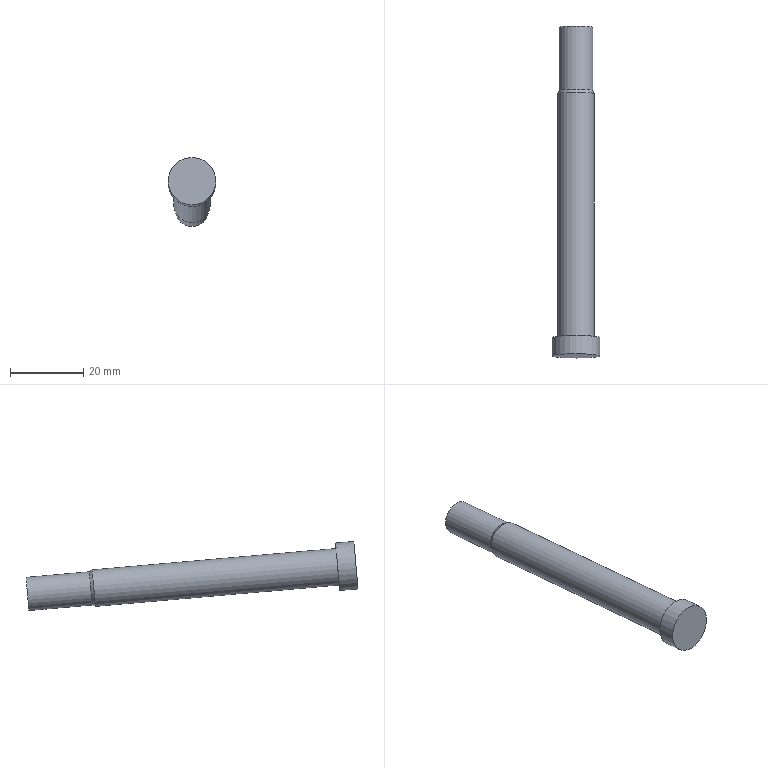Part | NX | features SPAS 10-80-7.100 2 | 1 solid | 7 faces | box 13 x 90.621 x 18.852 mm | volume 7099 mm3 | plane 3 | cylinder 3 | torus 1 | commonest cylinder face diameters 9.1 x1 10 x1 13 x1
STEP:
#1=CARTESIAN_POINT('',(-694.42,-51.795,-32.008));
#2=VERTEX_POINT('',#1);
#3=CARTESIAN_POINT('',(-694.42,-52.191,-36.54));
#4=DIRECTION('',(0.,0.9962,-0.08716));
#5=DIRECTION('',(0.,0.08716,0.9962));
#6=AXIS2_PLACEMENT_3D('',#3,#4,#5);
#7=CIRCLE('',#6,4.55);
#8=EDGE_CURVE('',#2,#2,#7,.F.);
#9=ORIENTED_EDGE('',*,*,#8,.F.);
#10=EDGE_LOOP('',(#9));
#11=FACE_BOUND('',#10,.T.);
#12=CARTESIAN_POINT('',(-694.42,-52.191,-36.54));
#13=DIRECTION('',(0.,0.9962,-0.08716));
#14=DIRECTION('',(0.,0.08716,0.9962));
#15=AXIS2_PLACEMENT_3D('',#12,#13,#14);
#16=PLANE('',#15);
#17=ADVANCED_FACE('',(#11),#16,.T.);
#18=CARTESIAN_POINT('',(-694.42,-69.087,-30.495));
#19=VERTEX_POINT('',#18);
#20=CARTESIAN_POINT('',(-694.42,-69.484,-35.027));
#21=DIRECTION('',(0.,0.9962,-0.08716));
#22=DIRECTION('',(0.,0.08716,0.9962));
#23=AXIS2_PLACEMENT_3D('',#20,#21,#22);
#24=CIRCLE('',#23,4.55);
#25=EDGE_CURVE('',#19,#19,#24,.T.);
#26=ORIENTED_EDGE('',*,*,#25,.T.);
#27=EDGE_LOOP('',(#26));
#28=FACE_BOUND('',#27,.T.);
#29=ORIENTED_EDGE('',*,*,#8,.T.);
#30=EDGE_LOOP('',(#29));
#31=FACE_BOUND('',#30,.T.);
#32=CARTESIAN_POINT('',(-694.42,-52.191,-36.54));
#33=DIRECTION('',(0.,-0.9962,0.08716));
#34=DIRECTION('',(0.,-0.08716,-0.9962));
#35=AXIS2_PLACEMENT_3D('',#32,#33,#34);
#36=CYLINDRICAL_SURFACE('',#35,4.55);
#37=ADVANCED_FACE('',(#28,#31),#36,.T.);
#38=CARTESIAN_POINT('',(-694.42,-136.432,-24.151));
#39=VERTEX_POINT('',#38);
#40=CARTESIAN_POINT('',(-694.42,-136.868,-29.132));
#41=DIRECTION('',(0.,0.9962,-0.08716));
#42=DIRECTION('',(0.,0.08716,0.9962));
#43=AXIS2_PLACEMENT_3D('',#40,#41,#42);
#44=CIRCLE('',#43,5.);
#45=EDGE_CURVE('',#39,#39,#44,.F.);
#46=ORIENTED_EDGE('',*,*,#45,.F.);
#47=EDGE_LOOP('',(#46));
#48=FACE_BOUND('',#47,.T.);
#49=CARTESIAN_POINT('',(-694.42,-70.744,-39.936));
#50=VERTEX_POINT('',#49);
#51=CARTESIAN_POINT('',(-694.42,-70.308,-34.955));
#52=DIRECTION('',(0.,-0.9962,0.08716));
#53=DIRECTION('',(0.,-0.08716,-0.9962));
#54=AXIS2_PLACEMENT_3D('',#51,#52,#53);
#55=CIRCLE('',#54,5.);
#56=EDGE_CURVE('',#50,#50,#55,.T.);
#57=ORIENTED_EDGE('',*,*,#56,.T.);
#58=EDGE_LOOP('',(#57));
#59=FACE_BOUND('',#58,.T.);
#60=CARTESIAN_POINT('',(-694.42,-70.308,-34.955));
#61=DIRECTION('',(0.,-0.9962,0.08716));
#62=DIRECTION('',(0.,-0.08716,-0.9962));
#63=AXIS2_PLACEMENT_3D('',#60,#61,#62);
#64=CYLINDRICAL_SURFACE('',#63,5.);
#65=ADVANCED_FACE('',(#48,#59),#64,.T.);
#66=CARTESIAN_POINT('',(-694.42,-142.415,-35.171));
#67=VERTEX_POINT('',#66);
#68=CARTESIAN_POINT('',(-694.42,-141.849,-28.696));
#69=DIRECTION('',(0.,-0.9962,0.08716));
#70=DIRECTION('',(0.,-0.08716,-0.9962));
#71=AXIS2_PLACEMENT_3D('',#68,#69,#70);
#72=CIRCLE('',#71,6.5);
#73=EDGE_CURVE('',#67,#67,#72,.F.);
#74=ORIENTED_EDGE('',*,*,#73,.F.);
#75=EDGE_LOOP('',(#74));
#76=FACE_BOUND('',#75,.T.);
#77=CARTESIAN_POINT('',(-694.42,-141.849,-28.696));
#78=DIRECTION('',(0.,-0.9962,0.08716));
#79=DIRECTION('',(0.,-0.08716,-0.9962));
#80=AXIS2_PLACEMENT_3D('',#77,#78,#79);
#81=PLANE('',#80);
#82=ADVANCED_FACE('',(#76),#81,.T.);
#83=ORIENTED_EDGE('',*,*,#45,.T.);
#84=EDGE_LOOP('',(#83));
#85=FACE_BOUND('',#84,.T.);
#86=CARTESIAN_POINT('',(-694.42,-136.301,-22.657));
#87=VERTEX_POINT('',#86);
#88=CARTESIAN_POINT('',(-694.42,-136.868,-29.132));
#89=DIRECTION('',(0.,0.9962,-0.08716));
#90=DIRECTION('',(0.,0.08716,0.9962));
#91=AXIS2_PLACEMENT_3D('',#88,#89,#90);
#92=CIRCLE('',#91,6.5);
#93=EDGE_CURVE('',#87,#87,#92,.F.);
#94=ORIENTED_EDGE('',*,*,#93,.F.);
#95=EDGE_LOOP('',(#94));
#96=FACE_BOUND('',#95,.T.);
#97=CARTESIAN_POINT('',(-694.42,-136.868,-29.132));
#98=DIRECTION('',(0.,0.9962,-0.08716));
#99=DIRECTION('',(0.,0.08716,0.9962));
#100=AXIS2_PLACEMENT_3D('',#97,#98,#99);
#101=PLANE('',#100);
#102=ADVANCED_FACE('',(#85,#96),#101,.T.);
#103=ORIENTED_EDGE('',*,*,#73,.T.);
#104=EDGE_LOOP('',(#103));
#105=FACE_BOUND('',#104,.T.);
#106=ORIENTED_EDGE('',*,*,#93,.T.);
#107=EDGE_LOOP('',(#106));
#108=FACE_BOUND('',#107,.T.);
#109=CARTESIAN_POINT('',(-694.42,-126.906,-30.004));
#110=DIRECTION('',(0.,-0.9962,0.08716));
#111=DIRECTION('',(0.,-0.08716,-0.9962));
#112=AXIS2_PLACEMENT_3D('',#109,#110,#111);
#113=CYLINDRICAL_SURFACE('',#112,6.5);
#114=ADVANCED_FACE('',(#105,#108),#113,.T.);
#115=ORIENTED_EDGE('',*,*,#25,.F.);
#116=EDGE_LOOP('',(#115));
#117=FACE_BOUND('',#116,.T.);
#118=ORIENTED_EDGE('',*,*,#56,.F.);
#119=EDGE_LOOP('',(#118));
#120=FACE_BOUND('',#119,.T.);
#121=CARTESIAN_POINT('',(-694.42,-65.142,-35.407));
#122=DIRECTION('',(0.,-0.9962,0.08716));
#123=DIRECTION('',(0.,-0.08716,-0.9962));
#124=AXIS2_PLACEMENT_3D('',#121,#122,#123);
#125=TOROIDAL_SURFACE('',#124,13.55,10.);
#126=ADVANCED_FACE('',(#117,#120),#125,.F.);
#127=CLOSED_SHELL('',(#17,#37,#65,#82,#102,#114,#126));
#128=MANIFOLD_SOLID_BREP('',#127);
#129=(LENGTH_UNIT()NAMED_UNIT(*)SI_UNIT(.MILLI.,.METRE.));
#130=UNCERTAINTY_MEASURE_WITH_UNIT(LENGTH_MEASURE(0.00001),#129,'','');
#131=(NAMED_UNIT(*)PLANE_ANGLE_UNIT()SI_UNIT($,.RADIAN.));
#132=(NAMED_UNIT(*)SI_UNIT($,.STERADIAN.)SOLID_ANGLE_UNIT());
#133=(GEOMETRIC_REPRESENTATION_CONTEXT(3)GLOBAL_UNCERTAINTY_ASSIGNED_CONTEXT((#130))GLOBAL_UNIT_ASSIGNED_CONTEXT((#129,#131,#132))REPRESENTATION_CONTEXT('',''));
#134=ADVANCED_BREP_SHAPE_REPRESENTATION('',(#128),#133);